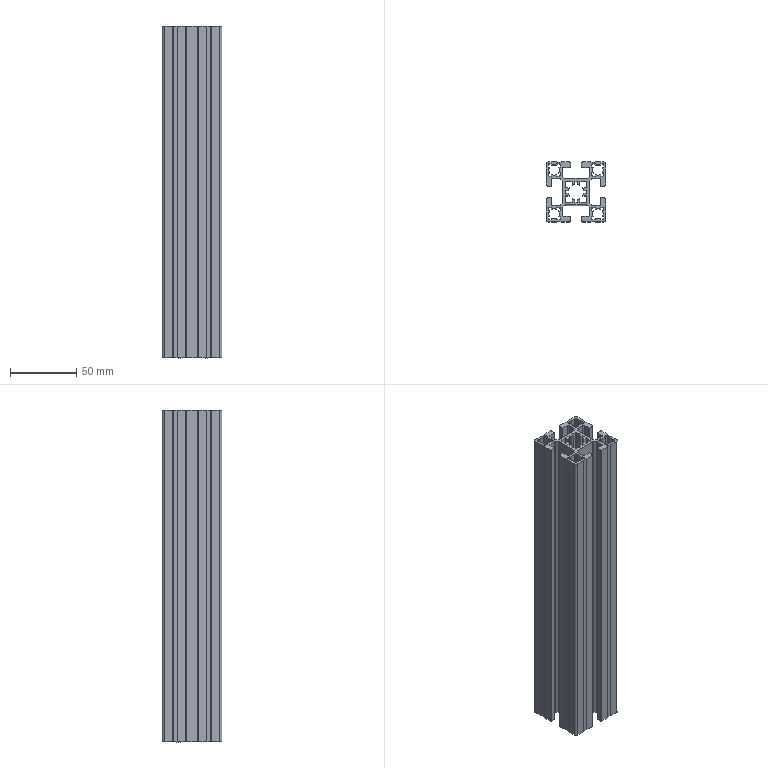Part | STEP file | 4545-250 | 1 solid | 262 faces | box 45 x 45 x 250 mm | volume 173462 mm3 | plane 186 | cylinder 76 | commonest cylinder face diameters 2 x44 8 x20 12 x8 4 x4